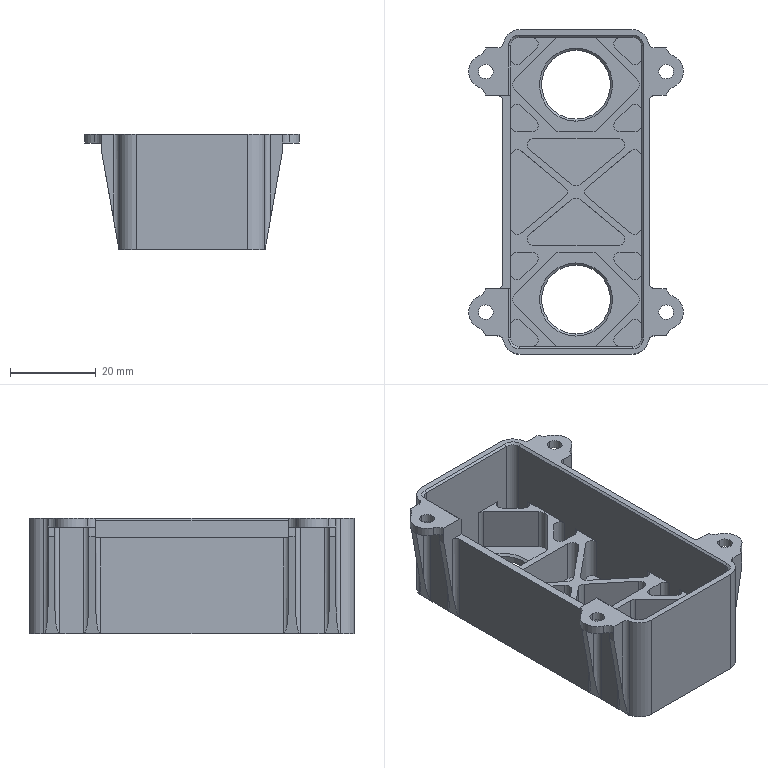NC program | NX | posted with a generic post | part box 50 x 75.58 x 26.8 mm
Lines 1 to 18 of 37241:
N10 G17 G21 G94 G90
(FLOOR_WALL_COPY , TOOL : D80)
N12 T19 M6
N14 G54
N16 G17 G0 G90 X-84.79 Y0. S6500 M3
N18 G43 Z30. H19
N20 Z3.
N22 G94 G1 Z0. F1500.
N24 X-79.79
N26 X79.79
N28 X84.79
N30 Z3.
N32 G0 Z30.
N34 M5